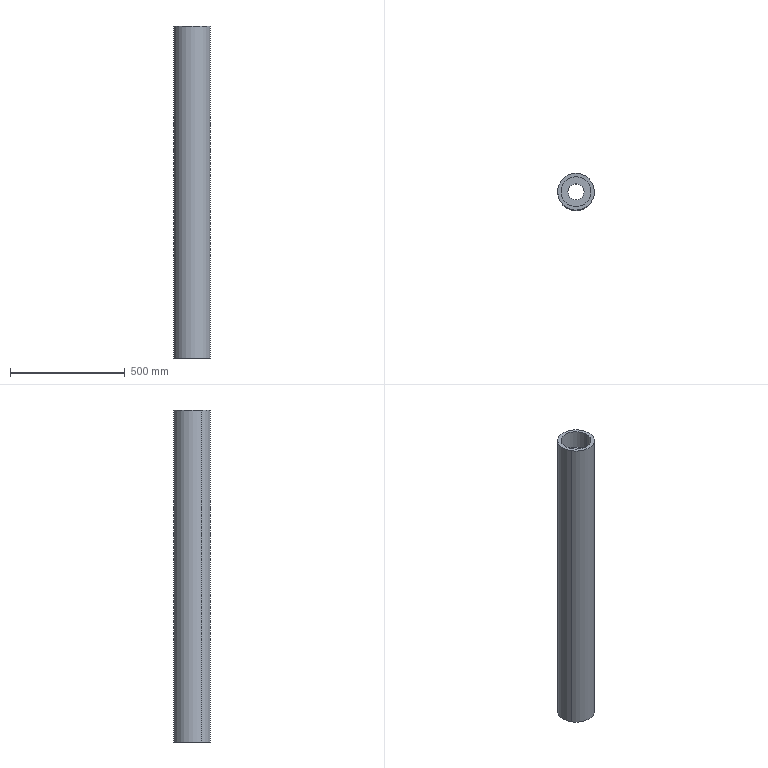Part | SolidWorks | features BaseBody 1 | 1 solid | 12 faces | box 160 x 160 x 1444 mm | volume 21949365 mm3 | cylinder 8 | plane 4 | commonest cylinder face diameters 130 x4 70 x2 160 x2
STEP:
#1=CARTESIAN_POINT('',(-126.923,853.249,-631.114));
#2=VERTEX_POINT('',#1);
#3=CARTESIAN_POINT('',(-126.923,853.249,-712.114));
#4=VERTEX_POINT('',#3);
#5=CARTESIAN_POINT('',(-126.923,853.249,-631.114));
#6=DIRECTION('',(0.,0.,-1.));
#7=VECTOR('',#6,1000.);
#8=LINE('',#5,#7);
#9=EDGE_CURVE('',#2,#4,#8,.T.);
#10=ORIENTED_EDGE('',*,*,#9,.F.);
#11=CARTESIAN_POINT('',(-256.923,853.249,-631.114));
#12=VERTEX_POINT('',#11);
#13=CARTESIAN_POINT('',(-191.923,853.249,-631.114));
#14=DIRECTION('',(0.,0.,1.));
#15=DIRECTION('',(0.,-1.,0.));
#16=AXIS2_PLACEMENT_3D('',#13,#14,#15);
#17=CIRCLE('',#16,65.);
#18=EDGE_CURVE('',#2,#12,#17,.T.);
#19=ORIENTED_EDGE('',*,*,#18,.T.);
#20=CARTESIAN_POINT('',(-256.923,853.249,-712.114));
#21=VERTEX_POINT('',#20);
#22=CARTESIAN_POINT('',(-256.923,853.249,-631.114));
#23=DIRECTION('',(0.,0.,-1.));
#24=VECTOR('',#23,1000.);
#25=LINE('',#22,#24);
#26=EDGE_CURVE('',#12,#21,#25,.T.);
#27=ORIENTED_EDGE('',*,*,#26,.T.);
#28=CARTESIAN_POINT('',(-191.923,853.249,-712.114));
#29=DIRECTION('',(0.,0.,1.));
#30=DIRECTION('',(-1.,0.,0.));
#31=AXIS2_PLACEMENT_3D('',#28,#29,#30);
#32=CIRCLE('',#31,65.);
#33=EDGE_CURVE('',#4,#21,#32,.T.);
#34=ORIENTED_EDGE('',*,*,#33,.F.);
#35=EDGE_LOOP('',(#10,#19,#27,#34));
#36=FACE_OUTER_BOUND('',#35,.T.);
#37=CARTESIAN_POINT('',(-191.923,853.249,-631.114));
#38=DIRECTION('',(0.,0.,-1.));
#39=DIRECTION('',(-1.,0.,0.));
#40=AXIS2_PLACEMENT_3D('',#37,#38,#39);
#41=CYLINDRICAL_SURFACE('',#40,65.);
#42=ADVANCED_FACE('',(#36),#41,.F.);
#43=CARTESIAN_POINT('',(-226.923,853.249,-631.114));
#44=VERTEX_POINT('',#43);
#45=CARTESIAN_POINT('',(-156.923,853.249,-631.114));
#46=VERTEX_POINT('',#45);
#47=CARTESIAN_POINT('',(-191.923,853.249,-631.114));
#48=DIRECTION('',(0.,0.,-1.));
#49=DIRECTION('',(1.,0.,0.));
#50=AXIS2_PLACEMENT_3D('',#47,#48,#49);
#51=CIRCLE('',#50,35.);
#52=EDGE_CURVE('',#44,#46,#51,.T.);
#53=ORIENTED_EDGE('',*,*,#52,.F.);
#54=CARTESIAN_POINT('',(-191.923,853.249,-631.114));
#55=DIRECTION('',(0.,0.,-1.));
#56=DIRECTION('',(1.,0.,0.));
#57=AXIS2_PLACEMENT_3D('',#54,#55,#56);
#58=CIRCLE('',#57,35.);
#59=EDGE_CURVE('',#46,#44,#58,.T.);
#60=ORIENTED_EDGE('',*,*,#59,.F.);
#61=EDGE_LOOP('',(#53,#60));
#62=FACE_BOUND('',#61,.T.);
#63=CARTESIAN_POINT('',(-191.923,853.249,-631.114));
#64=DIRECTION('',(0.,0.,1.));
#65=DIRECTION('',(0.,-1.,0.));
#66=AXIS2_PLACEMENT_3D('',#63,#64,#65);
#67=CIRCLE('',#66,65.);
#68=EDGE_CURVE('',#12,#2,#67,.T.);
#69=ORIENTED_EDGE('',*,*,#68,.F.);
#70=ORIENTED_EDGE('',*,*,#18,.F.);
#71=EDGE_LOOP('',(#69,#70));
#72=FACE_OUTER_BOUND('',#71,.T.);
#73=CARTESIAN_POINT('',(-191.923,853.249,-631.114));
#74=DIRECTION('',(0.,0.,1.));
#75=DIRECTION('',(1.,0.,0.));
#76=AXIS2_PLACEMENT_3D('',#73,#74,#75);
#77=PLANE('',#76);
#78=ADVANCED_FACE('',(#62,#72),#77,.F.);
#79=CARTESIAN_POINT('',(-226.923,853.249,650.886));
#80=VERTEX_POINT('',#79);
#81=CARTESIAN_POINT('',(-156.923,853.249,650.886));
#82=VERTEX_POINT('',#81);
#83=CARTESIAN_POINT('',(-191.923,853.249,650.886));
#84=DIRECTION('',(0.,0.,-1.));
#85=DIRECTION('',(1.,0.,0.));
#86=AXIS2_PLACEMENT_3D('',#83,#84,#85);
#87=CIRCLE('',#86,35.);
#88=EDGE_CURVE('',#80,#82,#87,.T.);
#89=ORIENTED_EDGE('',*,*,#88,.T.);
#90=CARTESIAN_POINT('',(-191.923,853.249,650.886));
#91=DIRECTION('',(0.,0.,-1.));
#92=DIRECTION('',(1.,0.,0.));
#93=AXIS2_PLACEMENT_3D('',#90,#91,#92);
#94=CIRCLE('',#93,35.);
#95=EDGE_CURVE('',#82,#80,#94,.T.);
#96=ORIENTED_EDGE('',*,*,#95,.T.);
#97=EDGE_LOOP('',(#89,#96));
#98=FACE_BOUND('',#97,.T.);
#99=CARTESIAN_POINT('',(-126.923,853.249,650.886));
#100=VERTEX_POINT('',#99);
#101=CARTESIAN_POINT('',(-256.923,853.249,650.886));
#102=VERTEX_POINT('',#101);
#103=CARTESIAN_POINT('',(-191.923,853.249,650.886));
#104=DIRECTION('',(0.,0.,1.));
#105=DIRECTION('',(0.,-1.,0.));
#106=AXIS2_PLACEMENT_3D('',#103,#104,#105);
#107=CIRCLE('',#106,65.);
#108=EDGE_CURVE('',#100,#102,#107,.T.);
#109=ORIENTED_EDGE('',*,*,#108,.T.);
#110=CARTESIAN_POINT('',(-191.923,853.249,650.886));
#111=DIRECTION('',(0.,0.,1.));
#112=DIRECTION('',(0.,-1.,0.));
#113=AXIS2_PLACEMENT_3D('',#110,#111,#112);
#114=CIRCLE('',#113,65.);
#115=EDGE_CURVE('',#102,#100,#114,.T.);
#116=ORIENTED_EDGE('',*,*,#115,.T.);
#117=EDGE_LOOP('',(#109,#116));
#118=FACE_OUTER_BOUND('',#117,.T.);
#119=CARTESIAN_POINT('',(-191.923,853.249,650.886));
#120=DIRECTION('',(0.,0.,1.));
#121=DIRECTION('',(1.,0.,0.));
#122=AXIS2_PLACEMENT_3D('',#119,#120,#121);
#123=PLANE('',#122);
#124=ADVANCED_FACE('',(#98,#118),#123,.T.);
#125=CARTESIAN_POINT('',(-256.923,853.249,731.886));
#126=VERTEX_POINT('',#125);
#127=CARTESIAN_POINT('',(-256.923,853.249,650.886));
#128=DIRECTION('',(0.,0.,1.));
#129=VECTOR('',#128,1000.);
#130=LINE('',#127,#129);
#131=EDGE_CURVE('',#102,#126,#130,.T.);
#132=ORIENTED_EDGE('',*,*,#131,.F.);
#133=ORIENTED_EDGE('',*,*,#108,.F.);
#134=CARTESIAN_POINT('',(-126.923,853.249,731.886));
#135=VERTEX_POINT('',#134);
#136=CARTESIAN_POINT('',(-126.923,853.249,650.886));
#137=DIRECTION('',(0.,0.,1.));
#138=VECTOR('',#137,1000.);
#139=LINE('',#136,#138);
#140=EDGE_CURVE('',#100,#135,#139,.T.);
#141=ORIENTED_EDGE('',*,*,#140,.T.);
#142=CARTESIAN_POINT('',(-191.923,853.249,731.886));
#143=DIRECTION('',(0.,0.,-1.));
#144=DIRECTION('',(-1.,0.,0.));
#145=AXIS2_PLACEMENT_3D('',#142,#143,#144);
#146=CIRCLE('',#145,65.);
#147=EDGE_CURVE('',#126,#135,#146,.T.);
#148=ORIENTED_EDGE('',*,*,#147,.F.);
#149=EDGE_LOOP('',(#132,#133,#141,#148));
#150=FACE_OUTER_BOUND('',#149,.T.);
#151=CARTESIAN_POINT('',(-191.923,853.249,650.886));
#152=DIRECTION('',(0.,0.,1.));
#153=DIRECTION('',(1.,0.,0.));
#154=AXIS2_PLACEMENT_3D('',#151,#152,#153);
#155=CYLINDRICAL_SURFACE('',#154,65.);
#156=ADVANCED_FACE('',(#150),#155,.F.);
#157=CARTESIAN_POINT('',(-260.497,812.048,-712.114));
#158=VERTEX_POINT('',#157);
#159=CARTESIAN_POINT('',(-260.497,812.048,731.886));
#160=VERTEX_POINT('',#159);
#161=CARTESIAN_POINT('',(-260.497,812.048,151.886));
#162=DIRECTION('',(0.,0.,1.));
#163=VECTOR('',#162,1000.);
#164=LINE('',#161,#163);
#165=EDGE_CURVE('',#158,#160,#164,.T.);
#166=ORIENTED_EDGE('',*,*,#165,.F.);
#167=CARTESIAN_POINT('',(-123.349,894.45,-712.114));
#168=VERTEX_POINT('',#167);
#169=CARTESIAN_POINT('',(-191.923,853.249,-712.114));
#170=DIRECTION('',(0.,0.,1.));
#171=DIRECTION('',(-1.,0.,0.));
#172=AXIS2_PLACEMENT_3D('',#169,#170,#171);
#173=CIRCLE('',#172,80.);
#174=EDGE_CURVE('',#158,#168,#173,.T.);
#175=ORIENTED_EDGE('',*,*,#174,.T.);
#176=CARTESIAN_POINT('',(-123.349,894.45,731.886));
#177=VERTEX_POINT('',#176);
#178=CARTESIAN_POINT('',(-123.349,894.45,151.886));
#179=DIRECTION('',(0.,0.,1.));
#180=VECTOR('',#179,1000.);
#181=LINE('',#178,#180);
#182=EDGE_CURVE('',#168,#177,#181,.T.);
#183=ORIENTED_EDGE('',*,*,#182,.T.);
#184=CARTESIAN_POINT('',(-191.923,853.249,731.886));
#185=DIRECTION('',(0.,0.,-1.));
#186=DIRECTION('',(-1.,0.,0.));
#187=AXIS2_PLACEMENT_3D('',#184,#185,#186);
#188=CIRCLE('',#187,80.);
#189=EDGE_CURVE('',#177,#160,#188,.T.);
#190=ORIENTED_EDGE('',*,*,#189,.T.);
#191=EDGE_LOOP('',(#166,#175,#183,#190));
#192=FACE_OUTER_BOUND('',#191,.T.);
#193=CARTESIAN_POINT('',(-191.923,853.249,151.886));
#194=DIRECTION('',(0.,0.,1.));
#195=DIRECTION('',(-0.8572,-0.515,0.));
#196=AXIS2_PLACEMENT_3D('',#193,#194,#195);
#197=CYLINDRICAL_SURFACE('',#196,80.);
#198=ADVANCED_FACE('',(#192),#197,.T.);
#199=ORIENTED_EDGE('',*,*,#182,.F.);
#200=CARTESIAN_POINT('',(-191.923,853.249,-712.114));
#201=DIRECTION('',(0.,0.,1.));
#202=DIRECTION('',(-1.,0.,0.));
#203=AXIS2_PLACEMENT_3D('',#200,#201,#202);
#204=CIRCLE('',#203,80.);
#205=EDGE_CURVE('',#168,#158,#204,.T.);
#206=ORIENTED_EDGE('',*,*,#205,.T.);
#207=ORIENTED_EDGE('',*,*,#165,.T.);
#208=CARTESIAN_POINT('',(-191.923,853.249,731.886));
#209=DIRECTION('',(0.,0.,-1.));
#210=DIRECTION('',(-1.,0.,0.));
#211=AXIS2_PLACEMENT_3D('',#208,#209,#210);
#212=CIRCLE('',#211,80.);
#213=EDGE_CURVE('',#160,#177,#212,.T.);
#214=ORIENTED_EDGE('',*,*,#213,.T.);
#215=EDGE_LOOP('',(#199,#206,#207,#214));
#216=FACE_OUTER_BOUND('',#215,.T.);
#217=CARTESIAN_POINT('',(-191.923,853.249,151.886));
#218=DIRECTION('',(0.,0.,1.));
#219=DIRECTION('',(-0.8572,-0.515,0.));
#220=AXIS2_PLACEMENT_3D('',#217,#218,#219);
#221=CYLINDRICAL_SURFACE('',#220,80.);
#222=ADVANCED_FACE('',(#216),#221,.T.);
#223=CARTESIAN_POINT('',(-191.923,853.249,731.886));
#224=DIRECTION('',(0.,0.,-1.));
#225=DIRECTION('',(-1.,0.,0.));
#226=AXIS2_PLACEMENT_3D('',#223,#224,#225);
#227=CIRCLE('',#226,65.);
#228=EDGE_CURVE('',#135,#126,#227,.T.);
#229=ORIENTED_EDGE('',*,*,#228,.T.);
#230=ORIENTED_EDGE('',*,*,#147,.T.);
#231=EDGE_LOOP('',(#229,#230));
#232=FACE_BOUND('',#231,.T.);
#233=ORIENTED_EDGE('',*,*,#213,.F.);
#234=ORIENTED_EDGE('',*,*,#189,.F.);
#235=EDGE_LOOP('',(#233,#234));
#236=FACE_OUTER_BOUND('',#235,.T.);
#237=CARTESIAN_POINT('',(-191.923,853.249,731.886));
#238=DIRECTION('',(0.,0.,-1.));
#239=DIRECTION('',(0.,-1.,0.));
#240=AXIS2_PLACEMENT_3D('',#237,#238,#239);
#241=PLANE('',#240);
#242=ADVANCED_FACE('',(#232,#236),#241,.F.);
#243=CARTESIAN_POINT('',(-156.923,853.249,1043.113));
#244=DIRECTION('',(0.,0.,-1.));
#245=VECTOR('',#244,1000.);
#246=LINE('',#243,#245);
#247=EDGE_CURVE('',#82,#46,#246,.T.);
#248=ORIENTED_EDGE('',*,*,#247,.F.);
#249=ORIENTED_EDGE('',*,*,#88,.F.);
#250=CARTESIAN_POINT('',(-226.923,853.249,1043.113));
#251=DIRECTION('',(0.,0.,-1.));
#252=VECTOR('',#251,1000.);
#253=LINE('',#250,#252);
#254=EDGE_CURVE('',#80,#44,#253,.T.);
#255=ORIENTED_EDGE('',*,*,#254,.T.);
#256=ORIENTED_EDGE('',*,*,#52,.T.);
#257=EDGE_LOOP('',(#248,#249,#255,#256));
#258=FACE_OUTER_BOUND('',#257,.T.);
#259=CARTESIAN_POINT('',(-191.923,853.249,1043.113));
#260=DIRECTION('',(0.,0.,-1.));
#261=DIRECTION('',(-1.,0.,0.));
#262=AXIS2_PLACEMENT_3D('',#259,#260,#261);
#263=CYLINDRICAL_SURFACE('',#262,35.);
#264=ADVANCED_FACE('',(#258),#263,.F.);
#265=CARTESIAN_POINT('',(-191.923,853.249,-712.114));
#266=DIRECTION('',(0.,0.,1.));
#267=DIRECTION('',(-1.,0.,0.));
#268=AXIS2_PLACEMENT_3D('',#265,#266,#267);
#269=CIRCLE('',#268,65.);
#270=EDGE_CURVE('',#21,#4,#269,.T.);
#271=ORIENTED_EDGE('',*,*,#270,.T.);
#272=ORIENTED_EDGE('',*,*,#33,.T.);
#273=EDGE_LOOP('',(#271,#272));
#274=FACE_BOUND('',#273,.T.);
#275=ORIENTED_EDGE('',*,*,#174,.F.);
#276=ORIENTED_EDGE('',*,*,#205,.F.);
#277=EDGE_LOOP('',(#275,#276));
#278=FACE_OUTER_BOUND('',#277,.T.);
#279=CARTESIAN_POINT('',(-191.923,853.249,-712.114));
#280=DIRECTION('',(0.,0.,-1.));
#281=DIRECTION('',(0.,-1.,0.));
#282=AXIS2_PLACEMENT_3D('',#279,#280,#281);
#283=PLANE('',#282);
#284=ADVANCED_FACE('',(#274,#278),#283,.T.);
#285=ORIENTED_EDGE('',*,*,#95,.F.);
#286=ORIENTED_EDGE('',*,*,#247,.T.);
#287=ORIENTED_EDGE('',*,*,#59,.T.);
#288=ORIENTED_EDGE('',*,*,#254,.F.);
#289=EDGE_LOOP('',(#285,#286,#287,#288));
#290=FACE_OUTER_BOUND('',#289,.T.);
#291=CARTESIAN_POINT('',(-191.923,853.249,1043.113));
#292=DIRECTION('',(0.,0.,-1.));
#293=DIRECTION('',(-1.,0.,0.));
#294=AXIS2_PLACEMENT_3D('',#291,#292,#293);
#295=CYLINDRICAL_SURFACE('',#294,35.);
#296=ADVANCED_FACE('',(#290),#295,.F.);
#297=ORIENTED_EDGE('',*,*,#115,.F.);
#298=ORIENTED_EDGE('',*,*,#131,.T.);
#299=ORIENTED_EDGE('',*,*,#228,.F.);
#300=ORIENTED_EDGE('',*,*,#140,.F.);
#301=EDGE_LOOP('',(#297,#298,#299,#300));
#302=FACE_OUTER_BOUND('',#301,.T.);
#303=CARTESIAN_POINT('',(-191.923,853.249,650.886));
#304=DIRECTION('',(0.,0.,1.));
#305=DIRECTION('',(1.,0.,0.));
#306=AXIS2_PLACEMENT_3D('',#303,#304,#305);
#307=CYLINDRICAL_SURFACE('',#306,65.);
#308=ADVANCED_FACE('',(#302),#307,.F.);
#309=ORIENTED_EDGE('',*,*,#68,.T.);
#310=ORIENTED_EDGE('',*,*,#9,.T.);
#311=ORIENTED_EDGE('',*,*,#270,.F.);
#312=ORIENTED_EDGE('',*,*,#26,.F.);
#313=EDGE_LOOP('',(#309,#310,#311,#312));
#314=FACE_OUTER_BOUND('',#313,.T.);
#315=CARTESIAN_POINT('',(-191.923,853.249,-631.114));
#316=DIRECTION('',(0.,0.,-1.));
#317=DIRECTION('',(-1.,0.,0.));
#318=AXIS2_PLACEMENT_3D('',#315,#316,#317);
#319=CYLINDRICAL_SURFACE('',#318,65.);
#320=ADVANCED_FACE('',(#314),#319,.F.);
#321=CLOSED_SHELL('',(#42,#78,#124,#156,#198,#222,#242,#264,#284,#296,#308,#320));
#322=MANIFOLD_SOLID_BREP('',#321);
#323=CARTESIAN_POINT('',(0.,0.,0.));
#324=DIRECTION('',(0.,0.,1.));
#325=DIRECTION('',(1.,0.,0.));
#326=AXIS2_PLACEMENT_3D('',#323,#324,#325);
#327=(LENGTH_UNIT()NAMED_UNIT(*)SI_UNIT(.MILLI.,.METRE.));
#328=UNCERTAINTY_MEASURE_WITH_UNIT(LENGTH_MEASURE(0.00001),#327,'','');
#329=(NAMED_UNIT(*)PLANE_ANGLE_UNIT()SI_UNIT($,.RADIAN.));
#330=(NAMED_UNIT(*)SI_UNIT($,.STERADIAN.)SOLID_ANGLE_UNIT());
#331=(GEOMETRIC_REPRESENTATION_CONTEXT(3)GLOBAL_UNCERTAINTY_ASSIGNED_CONTEXT((#328))GLOBAL_UNIT_ASSIGNED_CONTEXT((#327,#329,#330))REPRESENTATION_CONTEXT('',''));
#332=ADVANCED_BREP_SHAPE_REPRESENTATION('',(#322,#326),#331);